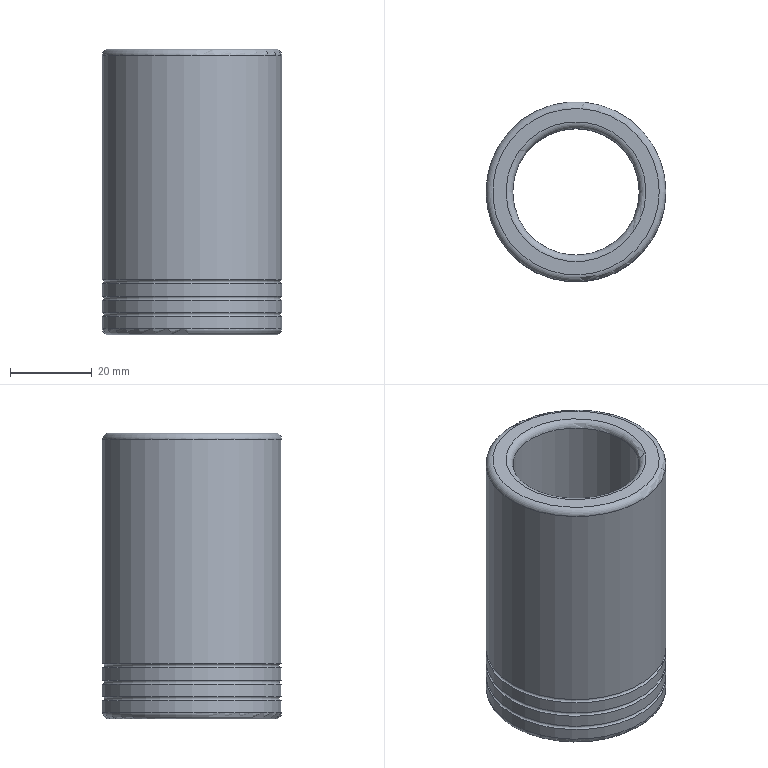Part | STEP file | 1 solid | 14 faces | box 44 x 44 x 70 mm | volume 53175 mm3 | torus 7 | cylinder 5 | plane 2 | commonest cylinder face diameters 44 x4 31 x1
STEP:
#1=CARTESIAN_POINT('',(0.,0.,0.));
#2=DIRECTION('',(0.,0.,1.));
#3=DIRECTION('',(1.,0.,0.));
#4=AXIS2_PLACEMENT_3D('',#1,#2,#3);
#5=CARTESIAN_POINT('',(1551.747,289.48,-77.006));
#6=VERTEX_POINT('',#5);
#7=CARTESIAN_POINT('',(1536.247,289.48,-77.006));
#8=DIRECTION('',(0.,0.,1.));
#9=DIRECTION('',(1.,0.,0.));
#10=AXIS2_PLACEMENT_3D('',#7,#8,#9);
#11=CIRCLE('',#10,15.5);
#12=CARTESIAN_POINT('',(1536.247,289.48,-125.381));
#13=DIRECTION('',(0.,0.,1.));
#14=DIRECTION('',(1.,0.,0.));
#15=AXIS2_PLACEMENT_3D('',#12,#13,#14);
#16=CYLINDRICAL_SURFACE('',#15,15.5);
#17=CARTESIAN_POINT('',(0.,48.375));
#18=DIRECTION('',(1.,0.));
#19=VECTOR('',#18,1.);
#20=LINE('',#17,#19);
#21=(GEOMETRIC_REPRESENTATION_CONTEXT(2)PARAMETRIC_REPRESENTATION_CONTEXT()REPRESENTATION_CONTEXT('',''));
#22=DEFINITIONAL_REPRESENTATION('',(#20),#21);
#23=PCURVE('',#16,#22);
#24=CARTESIAN_POINT('',(1536.247,289.48,-77.006));
#25=DIRECTION('',(0.,0.,1.));
#26=DIRECTION('',(1.,0.,0.));
#27=AXIS2_PLACEMENT_3D('',#24,#25,#26);
#28=TOROIDAL_SURFACE('',#27,17.125,1.625);
#29=CARTESIAN_POINT('',(0.,9.425));
#30=DIRECTION('',(1.,0.));
#31=VECTOR('',#30,1.);
#32=LINE('',#29,#31);
#33=(GEOMETRIC_REPRESENTATION_CONTEXT(2)PARAMETRIC_REPRESENTATION_CONTEXT()REPRESENTATION_CONTEXT('',''));
#34=DEFINITIONAL_REPRESENTATION('',(#32),#33);
#35=PCURVE('',#28,#34);
#36=SURFACE_CURVE('',#11,(#23,#35),.PCURVE_S1.);
#37=EDGE_CURVE('',#6,#6,#36,.T.);
#38=ORIENTED_EDGE('',*,*,#37,.F.);
#39=CARTESIAN_POINT('',(1551.747,289.48,-143.756));
#40=VERTEX_POINT('',#39);
#41=CARTESIAN_POINT('',(1551.747,289.48,-143.756));
#42=CARTESIAN_POINT('',(1551.747,289.48,-77.006));
#43=B_SPLINE_CURVE_WITH_KNOTS('',1,(#41,#42),.UNSPECIFIED.,.F.,.F.,(2,2),(-18.375,48.375),.PIECEWISE_BEZIER_KNOTS.);
#44=CARTESIAN_POINT('',(0.,0.));
#45=DIRECTION('',(0.,1.));
#46=VECTOR('',#45,1.);
#47=LINE('',#44,#46);
#48=(GEOMETRIC_REPRESENTATION_CONTEXT(2)PARAMETRIC_REPRESENTATION_CONTEXT()REPRESENTATION_CONTEXT('',''));
#49=DEFINITIONAL_REPRESENTATION('',(#47),#48);
#50=PCURVE('',#16,#49);
#51=CARTESIAN_POINT('',(6.283,0.));
#52=DIRECTION('',(0.,1.));
#53=VECTOR('',#52,1.);
#54=LINE('',#51,#53);
#55=(GEOMETRIC_REPRESENTATION_CONTEXT(2)PARAMETRIC_REPRESENTATION_CONTEXT()REPRESENTATION_CONTEXT('',''));
#56=DEFINITIONAL_REPRESENTATION('',(#54),#55);
#57=PCURVE('',#16,#56);
#58=SEAM_CURVE('',#43,(#50,#57),.PCURVE_S1.);
#59=EDGE_CURVE('',#40,#6,#58,.T.);
#60=ORIENTED_EDGE('',*,*,#59,.F.);
#61=CARTESIAN_POINT('',(1520.747,289.48,-143.756));
#62=VERTEX_POINT('',#61);
#63=CARTESIAN_POINT('',(1536.247,289.48,-143.756));
#64=DIRECTION('',(0.,0.,-1.));
#65=DIRECTION('',(-1.,0.,0.));
#66=AXIS2_PLACEMENT_3D('',#63,#64,#65);
#67=CIRCLE('',#66,15.5);
#68=CARTESIAN_POINT('',(3.142,-18.375));
#69=DIRECTION('',(-1.,0.));
#70=VECTOR('',#69,1.);
#71=LINE('',#68,#70);
#72=(GEOMETRIC_REPRESENTATION_CONTEXT(2)PARAMETRIC_REPRESENTATION_CONTEXT()REPRESENTATION_CONTEXT('',''));
#73=DEFINITIONAL_REPRESENTATION('',(#71),#72);
#74=PCURVE('',#16,#73);
#75=CARTESIAN_POINT('',(1536.247,289.48,-143.756));
#76=DIRECTION('',(0.,0.,-1.));
#77=DIRECTION('',(-1.,0.,0.));
#78=AXIS2_PLACEMENT_3D('',#75,#76,#77);
#79=TOROIDAL_SURFACE('',#78,17.125,1.625);
#80=CARTESIAN_POINT('',(0.,9.425));
#81=DIRECTION('',(1.,0.));
#82=VECTOR('',#81,1.);
#83=LINE('',#80,#82);
#84=(GEOMETRIC_REPRESENTATION_CONTEXT(2)PARAMETRIC_REPRESENTATION_CONTEXT()REPRESENTATION_CONTEXT('',''));
#85=DEFINITIONAL_REPRESENTATION('',(#83),#84);
#86=PCURVE('',#79,#85);
#87=SURFACE_CURVE('',#67,(#74,#86),.PCURVE_S1.);
#88=EDGE_CURVE('',#62,#40,#87,.T.);
#89=ORIENTED_EDGE('',*,*,#88,.F.);
#90=CARTESIAN_POINT('',(1536.247,289.48,-143.756));
#91=DIRECTION('',(0.,0.,-1.));
#92=DIRECTION('',(-1.,0.,0.));
#93=AXIS2_PLACEMENT_3D('',#90,#91,#92);
#94=CIRCLE('',#93,15.5);
#95=CARTESIAN_POINT('',(9.425,-18.375));
#96=DIRECTION('',(-1.,0.));
#97=VECTOR('',#96,1.);
#98=LINE('',#95,#97);
#99=(GEOMETRIC_REPRESENTATION_CONTEXT(2)PARAMETRIC_REPRESENTATION_CONTEXT()REPRESENTATION_CONTEXT('',''));
#100=DEFINITIONAL_REPRESENTATION('',(#98),#99);
#101=PCURVE('',#16,#100);
#102=CARTESIAN_POINT('',(0.,9.425));
#103=DIRECTION('',(1.,0.));
#104=VECTOR('',#103,1.);
#105=LINE('',#102,#104);
#106=(GEOMETRIC_REPRESENTATION_CONTEXT(2)PARAMETRIC_REPRESENTATION_CONTEXT()REPRESENTATION_CONTEXT('',''));
#107=DEFINITIONAL_REPRESENTATION('',(#105),#106);
#108=PCURVE('',#79,#107);
#109=SURFACE_CURVE('',#94,(#101,#108),.PCURVE_S1.);
#110=EDGE_CURVE('',#40,#62,#109,.T.);
#111=ORIENTED_EDGE('',*,*,#110,.F.);
#112=ORIENTED_EDGE('',*,*,#59,.T.);
#113=EDGE_LOOP('',(#38,#60,#89,#111,#112));
#114=FACE_BOUND('',#113,.F.);
#115=ADVANCED_FACE('',(#114),#16,.F.);
#116=CARTESIAN_POINT('',(1553.372,289.48,-75.381));
#117=VERTEX_POINT('',#116);
#118=CARTESIAN_POINT('',(1536.247,289.48,-75.381));
#119=DIRECTION('',(0.,0.,-1.));
#120=DIRECTION('',(1.,0.,0.));
#121=AXIS2_PLACEMENT_3D('',#118,#119,#120);
#122=CIRCLE('',#121,17.125);
#123=CARTESIAN_POINT('',(1520.747,289.48,-75.381));
#124=DIRECTION('',(0.,0.,1.));
#125=DIRECTION('',(1.,0.,0.));
#126=AXIS2_PLACEMENT_3D('',#123,#124,#125);
#127=PLANE('',#126);
#128=CARTESIAN_POINT('',(32.625,0.));
#129=CARTESIAN_POINT('',(32.625,-29.661));
#130=CARTESIAN_POINT('',(6.938,-14.831));
#131=CARTESIAN_POINT('',(-18.75,0.));
#132=CARTESIAN_POINT('',(6.938,14.831));
#133=CARTESIAN_POINT('',(32.625,29.661));
#134=CARTESIAN_POINT('',(32.625,0.));
#135=(BOUNDED_CURVE()B_SPLINE_CURVE(2,(#128,#129,#130,#131,#132,#133,#134),.UNSPECIFIED.,.T.,.F.)B_SPLINE_CURVE_WITH_KNOTS((1,2,2,2,2,1),(-2.094,0.,2.094,4.189,6.283,8.378),.UNSPECIFIED.)CURVE()GEOMETRIC_REPRESENTATION_ITEM()RATIONAL_B_SPLINE_CURVE((1.,0.5,1.,0.5,1.,0.5,1.))REPRESENTATION_ITEM(''));
#136=(GEOMETRIC_REPRESENTATION_CONTEXT(2)PARAMETRIC_REPRESENTATION_CONTEXT()REPRESENTATION_CONTEXT('',''));
#137=DEFINITIONAL_REPRESENTATION('',(#135),#136);
#138=PCURVE('',#127,#137);
#139=CARTESIAN_POINT('',(6.283,7.854));
#140=DIRECTION('',(-1.,0.));
#141=VECTOR('',#140,1.);
#142=LINE('',#139,#141);
#143=(GEOMETRIC_REPRESENTATION_CONTEXT(2)PARAMETRIC_REPRESENTATION_CONTEXT()REPRESENTATION_CONTEXT('',''));
#144=DEFINITIONAL_REPRESENTATION('',(#142),#143);
#145=PCURVE('',#28,#144);
#146=SURFACE_CURVE('',#122,(#138,#145),.PCURVE_S1.);
#147=EDGE_CURVE('',#117,#117,#146,.T.);
#148=ORIENTED_EDGE('',*,*,#147,.T.);
#149=EDGE_LOOP('',(#148));
#150=FACE_BOUND('',#149,.T.);
#151=CARTESIAN_POINT('',(1556.622,289.48,-75.381));
#152=VERTEX_POINT('',#151);
#153=CARTESIAN_POINT('',(1536.247,289.48,-75.381));
#154=DIRECTION('',(0.,0.,1.));
#155=DIRECTION('',(1.,0.,0.));
#156=AXIS2_PLACEMENT_3D('',#153,#154,#155);
#157=CIRCLE('',#156,20.375);
#158=CARTESIAN_POINT('',(15.5,0.));
#159=DIRECTION('',(1.,0.));
#160=AXIS2_PLACEMENT_2D('',#158,#159);
#161=CIRCLE('',#160,20.375);
#162=(GEOMETRIC_REPRESENTATION_CONTEXT(2)PARAMETRIC_REPRESENTATION_CONTEXT()REPRESENTATION_CONTEXT('',''));
#163=DEFINITIONAL_REPRESENTATION('',(#161),#162);
#164=PCURVE('',#127,#163);
#165=CARTESIAN_POINT('',(1536.247,289.48,-77.006));
#166=DIRECTION('',(0.,0.,1.));
#167=DIRECTION('',(1.,0.,0.));
#168=AXIS2_PLACEMENT_3D('',#165,#166,#167);
#169=TOROIDAL_SURFACE('',#168,20.375,1.625);
#170=CARTESIAN_POINT('',(0.,7.854));
#171=DIRECTION('',(1.,0.));
#172=VECTOR('',#171,1.);
#173=LINE('',#170,#172);
#174=(GEOMETRIC_REPRESENTATION_CONTEXT(2)PARAMETRIC_REPRESENTATION_CONTEXT()REPRESENTATION_CONTEXT('',''));
#175=DEFINITIONAL_REPRESENTATION('',(#173),#174);
#176=PCURVE('',#169,#175);
#177=SURFACE_CURVE('',#157,(#164,#176),.PCURVE_S1.);
#178=EDGE_CURVE('',#152,#152,#177,.T.);
#179=ORIENTED_EDGE('',*,*,#178,.T.);
#180=EDGE_LOOP('',(#179));
#181=FACE_BOUND('',#180,.T.);
#182=ADVANCED_FACE('',(#150,#181),#127,.T.);
#183=CARTESIAN_POINT('',(1558.247,289.48,-77.006));
#184=VERTEX_POINT('',#183);
#185=CARTESIAN_POINT('',(1536.247,289.48,-77.006));
#186=DIRECTION('',(0.,0.,-1.));
#187=DIRECTION('',(1.,0.,0.));
#188=AXIS2_PLACEMENT_3D('',#185,#186,#187);
#189=CIRCLE('',#188,22.);
#190=CARTESIAN_POINT('',(1536.247,289.48,-125.381));
#191=DIRECTION('',(0.,0.,1.));
#192=DIRECTION('',(1.,0.,0.));
#193=AXIS2_PLACEMENT_3D('',#190,#191,#192);
#194=CYLINDRICAL_SURFACE('',#193,22.);
#195=CARTESIAN_POINT('',(6.283,48.375));
#196=DIRECTION('',(-1.,0.));
#197=VECTOR('',#196,1.);
#198=LINE('',#195,#197);
#199=(GEOMETRIC_REPRESENTATION_CONTEXT(2)PARAMETRIC_REPRESENTATION_CONTEXT()REPRESENTATION_CONTEXT('',''));
#200=DEFINITIONAL_REPRESENTATION('',(#198),#199);
#201=PCURVE('',#194,#200);
#202=CARTESIAN_POINT('',(6.283,6.283));
#203=DIRECTION('',(-1.,0.));
#204=VECTOR('',#203,1.);
#205=LINE('',#202,#204);
#206=(GEOMETRIC_REPRESENTATION_CONTEXT(2)PARAMETRIC_REPRESENTATION_CONTEXT()REPRESENTATION_CONTEXT('',''));
#207=DEFINITIONAL_REPRESENTATION('',(#205),#206);
#208=PCURVE('',#169,#207);
#209=SURFACE_CURVE('',#189,(#201,#208),.PCURVE_S1.);
#210=EDGE_CURVE('',#184,#184,#209,.T.);
#211=ORIENTED_EDGE('',*,*,#210,.T.);
#212=CARTESIAN_POINT('',(1558.247,289.48,-131.881));
#213=VERTEX_POINT('',#212);
#214=CARTESIAN_POINT('',(1558.247,289.48,-131.881));
#215=CARTESIAN_POINT('',(1558.247,289.48,-77.006));
#216=B_SPLINE_CURVE_WITH_KNOTS('',1,(#214,#215),.UNSPECIFIED.,.F.,.F.,(2,2),(-6.5,48.375),.PIECEWISE_BEZIER_KNOTS.);
#217=CARTESIAN_POINT('',(0.,0.));
#218=DIRECTION('',(0.,1.));
#219=VECTOR('',#218,1.);
#220=LINE('',#217,#219);
#221=(GEOMETRIC_REPRESENTATION_CONTEXT(2)PARAMETRIC_REPRESENTATION_CONTEXT()REPRESENTATION_CONTEXT('',''));
#222=DEFINITIONAL_REPRESENTATION('',(#220),#221);
#223=PCURVE('',#194,#222);
#224=CARTESIAN_POINT('',(6.283,0.));
#225=DIRECTION('',(0.,1.));
#226=VECTOR('',#225,1.);
#227=LINE('',#224,#226);
#228=(GEOMETRIC_REPRESENTATION_CONTEXT(2)PARAMETRIC_REPRESENTATION_CONTEXT()REPRESENTATION_CONTEXT('',''));
#229=DEFINITIONAL_REPRESENTATION('',(#227),#228);
#230=PCURVE('',#194,#229);
#231=SEAM_CURVE('',#216,(#223,#230),.PCURVE_S1.);
#232=EDGE_CURVE('',#213,#184,#231,.T.);
#233=ORIENTED_EDGE('',*,*,#232,.F.);
#234=CARTESIAN_POINT('',(1536.247,289.48,-131.881));
#235=DIRECTION('',(0.,0.,1.));
#236=DIRECTION('',(1.,0.,0.));
#237=AXIS2_PLACEMENT_3D('',#234,#235,#236);
#238=CIRCLE('',#237,22.);
#239=CARTESIAN_POINT('',(0.,-6.5));
#240=DIRECTION('',(1.,0.));
#241=VECTOR('',#240,1.);
#242=LINE('',#239,#241);
#243=(GEOMETRIC_REPRESENTATION_CONTEXT(2)PARAMETRIC_REPRESENTATION_CONTEXT()REPRESENTATION_CONTEXT('',''));
#244=DEFINITIONAL_REPRESENTATION('',(#242),#243);
#245=PCURVE('',#194,#244);
#246=CARTESIAN_POINT('',(1536.247,289.48,-132.381));
#247=DIRECTION('',(0.,0.,1.));
#248=DIRECTION('',(1.,0.,0.));
#249=AXIS2_PLACEMENT_3D('',#246,#247,#248);
#250=TOROIDAL_SURFACE('',#249,22.,0.5);
#251=CARTESIAN_POINT('',(0.,1.571));
#252=DIRECTION('',(1.,0.));
#253=VECTOR('',#252,1.);
#254=LINE('',#251,#253);
#255=(GEOMETRIC_REPRESENTATION_CONTEXT(2)PARAMETRIC_REPRESENTATION_CONTEXT()REPRESENTATION_CONTEXT('',''));
#256=DEFINITIONAL_REPRESENTATION('',(#254),#255);
#257=PCURVE('',#250,#256);
#258=SURFACE_CURVE('',#238,(#245,#257),.PCURVE_S1.);
#259=EDGE_CURVE('',#213,#213,#258,.T.);
#260=ORIENTED_EDGE('',*,*,#259,.T.);
#261=ORIENTED_EDGE('',*,*,#232,.T.);
#262=EDGE_LOOP('',(#211,#233,#260,#261));
#263=FACE_BOUND('',#262,.T.);
#264=ADVANCED_FACE('',(#263),#194,.T.);
#265=CARTESIAN_POINT('',(1558.247,289.48,-132.881));
#266=VERTEX_POINT('',#265);
#267=CARTESIAN_POINT('',(1536.247,289.48,-132.881));
#268=DIRECTION('',(0.,0.,1.));
#269=DIRECTION('',(1.,0.,0.));
#270=AXIS2_PLACEMENT_3D('',#267,#268,#269);
#271=CIRCLE('',#270,22.);
#272=CARTESIAN_POINT('',(0.,4.712));
#273=DIRECTION('',(1.,0.));
#274=VECTOR('',#273,1.);
#275=LINE('',#272,#274);
#276=(GEOMETRIC_REPRESENTATION_CONTEXT(2)PARAMETRIC_REPRESENTATION_CONTEXT()REPRESENTATION_CONTEXT('',''));
#277=DEFINITIONAL_REPRESENTATION('',(#275),#276);
#278=PCURVE('',#250,#277);
#279=CARTESIAN_POINT('',(1536.247,289.48,-125.381));
#280=DIRECTION('',(0.,0.,1.));
#281=DIRECTION('',(1.,0.,0.));
#282=AXIS2_PLACEMENT_3D('',#279,#280,#281);
#283=CYLINDRICAL_SURFACE('',#282,22.);
#284=CARTESIAN_POINT('',(0.,-7.5));
#285=DIRECTION('',(1.,0.));
#286=VECTOR('',#285,1.);
#287=LINE('',#284,#286);
#288=(GEOMETRIC_REPRESENTATION_CONTEXT(2)PARAMETRIC_REPRESENTATION_CONTEXT()REPRESENTATION_CONTEXT('',''));
#289=DEFINITIONAL_REPRESENTATION('',(#287),#288);
#290=PCURVE('',#283,#289);
#291=SURFACE_CURVE('',#271,(#278,#290),.PCURVE_S1.);
#292=EDGE_CURVE('',#266,#266,#291,.T.);
#293=ORIENTED_EDGE('',*,*,#292,.F.);
#294=CARTESIAN_POINT('',(1558.247,289.48,-131.881));
#295=CARTESIAN_POINT('',(1558.023,289.48,-131.881));
#296=CARTESIAN_POINT('',(1557.799,289.48,-131.998));
#297=CARTESIAN_POINT('',(1557.647,289.48,-132.233));
#298=CARTESIAN_POINT('',(1557.647,289.48,-132.529));
#299=CARTESIAN_POINT('',(1557.799,289.48,-132.763));
#300=CARTESIAN_POINT('',(1558.023,289.48,-132.881));
#301=CARTESIAN_POINT('',(1558.247,289.48,-132.881));
#302=B_SPLINE_CURVE_WITH_KNOTS('',7,(#294,#295,#296,#297,#298,#299,#300,#301),.UNSPECIFIED.,.F.,.F.,(8,8),(1.571,4.712),.PIECEWISE_BEZIER_KNOTS.);
#303=CARTESIAN_POINT('',(0.,0.));
#304=DIRECTION('',(0.,1.));
#305=VECTOR('',#304,1.);
#306=LINE('',#303,#305);
#307=(GEOMETRIC_REPRESENTATION_CONTEXT(2)PARAMETRIC_REPRESENTATION_CONTEXT()REPRESENTATION_CONTEXT('',''));
#308=DEFINITIONAL_REPRESENTATION('',(#306),#307);
#309=PCURVE('',#250,#308);
#310=CARTESIAN_POINT('',(6.283,0.));
#311=DIRECTION('',(0.,1.));
#312=VECTOR('',#311,1.);
#313=LINE('',#310,#312);
#314=(GEOMETRIC_REPRESENTATION_CONTEXT(2)PARAMETRIC_REPRESENTATION_CONTEXT()REPRESENTATION_CONTEXT('',''));
#315=DEFINITIONAL_REPRESENTATION('',(#313),#314);
#316=PCURVE('',#250,#315);
#317=SEAM_CURVE('',#302,(#309,#316),.PCURVE_S1.);
#318=EDGE_CURVE('',#213,#266,#317,.T.);
#319=ORIENTED_EDGE('',*,*,#318,.F.);
#320=ORIENTED_EDGE('',*,*,#259,.T.);
#321=ORIENTED_EDGE('',*,*,#318,.T.);
#322=EDGE_LOOP('',(#293,#319,#320,#321));
#323=FACE_BOUND('',#322,.F.);
#324=ADVANCED_FACE('',(#323),#250,.F.);
#325=CARTESIAN_POINT('',(1558.247,289.48,-135.881));
#326=VERTEX_POINT('',#325);
#327=CARTESIAN_POINT('',(1536.247,289.48,-135.881));
#328=DIRECTION('',(0.,0.,1.));
#329=DIRECTION('',(1.,0.,0.));
#330=AXIS2_PLACEMENT_3D('',#327,#328,#329);
#331=CIRCLE('',#330,22.);
#332=CARTESIAN_POINT('',(0.,-10.5));
#333=DIRECTION('',(1.,0.));
#334=VECTOR('',#333,1.);
#335=LINE('',#332,#334);
#336=(GEOMETRIC_REPRESENTATION_CONTEXT(2)PARAMETRIC_REPRESENTATION_CONTEXT()REPRESENTATION_CONTEXT('',''));
#337=DEFINITIONAL_REPRESENTATION('',(#335),#336);
#338=PCURVE('',#283,#337);
#339=CARTESIAN_POINT('',(1536.247,289.48,-136.381));
#340=DIRECTION('',(0.,0.,1.));
#341=DIRECTION('',(1.,0.,0.));
#342=AXIS2_PLACEMENT_3D('',#339,#340,#341);
#343=TOROIDAL_SURFACE('',#342,22.,0.5);
#344=CARTESIAN_POINT('',(0.,1.571));
#345=DIRECTION('',(1.,0.));
#346=VECTOR('',#345,1.);
#347=LINE('',#344,#346);
#348=(GEOMETRIC_REPRESENTATION_CONTEXT(2)PARAMETRIC_REPRESENTATION_CONTEXT()REPRESENTATION_CONTEXT('',''));
#349=DEFINITIONAL_REPRESENTATION('',(#347),#348);
#350=PCURVE('',#343,#349);
#351=SURFACE_CURVE('',#331,(#338,#350),.PCURVE_S1.);
#352=EDGE_CURVE('',#326,#326,#351,.T.);
#353=ORIENTED_EDGE('',*,*,#352,.T.);
#354=CARTESIAN_POINT('',(1558.247,289.48,-135.881));
#355=CARTESIAN_POINT('',(1558.247,289.48,-132.881));
#356=B_SPLINE_CURVE_WITH_KNOTS('',1,(#354,#355),.UNSPECIFIED.,.F.,.F.,(2,2),(-10.5,-7.5),.PIECEWISE_BEZIER_KNOTS.);
#357=CARTESIAN_POINT('',(6.283,0.));
#358=DIRECTION('',(0.,1.));
#359=VECTOR('',#358,1.);
#360=LINE('',#357,#359);
#361=(GEOMETRIC_REPRESENTATION_CONTEXT(2)PARAMETRIC_REPRESENTATION_CONTEXT()REPRESENTATION_CONTEXT('',''));
#362=DEFINITIONAL_REPRESENTATION('',(#360),#361);
#363=PCURVE('',#283,#362);
#364=CARTESIAN_POINT('',(0.,0.));
#365=DIRECTION('',(0.,1.));
#366=VECTOR('',#365,1.);
#367=LINE('',#364,#366);
#368=(GEOMETRIC_REPRESENTATION_CONTEXT(2)PARAMETRIC_REPRESENTATION_CONTEXT()REPRESENTATION_CONTEXT('',''));
#369=DEFINITIONAL_REPRESENTATION('',(#367),#368);
#370=PCURVE('',#283,#369);
#371=SEAM_CURVE('',#356,(#363,#370),.PCURVE_S1.);
#372=EDGE_CURVE('',#326,#266,#371,.T.);
#373=ORIENTED_EDGE('',*,*,#372,.T.);
#374=ORIENTED_EDGE('',*,*,#292,.F.);
#375=ORIENTED_EDGE('',*,*,#372,.F.);
#376=EDGE_LOOP('',(#353,#373,#374,#375));
#377=FACE_BOUND('',#376,.T.);
#378=ADVANCED_FACE('',(#377),#283,.T.);
#379=CARTESIAN_POINT('',(1558.247,289.48,-136.881));
#380=VERTEX_POINT('',#379);
#381=CARTESIAN_POINT('',(1536.247,289.48,-136.881));
#382=DIRECTION('',(0.,0.,1.));
#383=DIRECTION('',(1.,0.,0.));
#384=AXIS2_PLACEMENT_3D('',#381,#382,#383);
#385=CIRCLE('',#384,22.);
#386=CARTESIAN_POINT('',(0.,4.712));
#387=DIRECTION('',(1.,0.));
#388=VECTOR('',#387,1.);
#389=LINE('',#386,#388);
#390=(GEOMETRIC_REPRESENTATION_CONTEXT(2)PARAMETRIC_REPRESENTATION_CONTEXT()REPRESENTATION_CONTEXT('',''));
#391=DEFINITIONAL_REPRESENTATION('',(#389),#390);
#392=PCURVE('',#343,#391);
#393=CARTESIAN_POINT('',(1536.247,289.48,-125.381));
#394=DIRECTION('',(0.,0.,1.));
#395=DIRECTION('',(1.,0.,0.));
#396=AXIS2_PLACEMENT_3D('',#393,#394,#395);
#397=CYLINDRICAL_SURFACE('',#396,22.);
#398=CARTESIAN_POINT('',(0.,-11.5));
#399=DIRECTION('',(1.,0.));
#400=VECTOR('',#399,1.);
#401=LINE('',#398,#400);
#402=(GEOMETRIC_REPRESENTATION_CONTEXT(2)PARAMETRIC_REPRESENTATION_CONTEXT()REPRESENTATION_CONTEXT('',''));
#403=DEFINITIONAL_REPRESENTATION('',(#401),#402);
#404=PCURVE('',#397,#403);
#405=SURFACE_CURVE('',#385,(#392,#404),.PCURVE_S1.);
#406=EDGE_CURVE('',#380,#380,#405,.T.);
#407=ORIENTED_EDGE('',*,*,#406,.F.);
#408=CARTESIAN_POINT('',(1558.247,289.48,-135.881));
#409=CARTESIAN_POINT('',(1558.023,289.48,-135.881));
#410=CARTESIAN_POINT('',(1557.799,289.48,-135.998));
#411=CARTESIAN_POINT('',(1557.647,289.48,-136.233));
#412=CARTESIAN_POINT('',(1557.647,289.48,-136.529));
#413=CARTESIAN_POINT('',(1557.799,289.48,-136.763));
#414=CARTESIAN_POINT('',(1558.023,289.48,-136.881));
#415=CARTESIAN_POINT('',(1558.247,289.48,-136.881));
#416=B_SPLINE_CURVE_WITH_KNOTS('',7,(#408,#409,#410,#411,#412,#413,#414,#415),.UNSPECIFIED.,.F.,.F.,(8,8),(1.571,4.712),.PIECEWISE_BEZIER_KNOTS.);
#417=CARTESIAN_POINT('',(0.,0.));
#418=DIRECTION('',(0.,1.));
#419=VECTOR('',#418,1.);
#420=LINE('',#417,#419);
#421=(GEOMETRIC_REPRESENTATION_CONTEXT(2)PARAMETRIC_REPRESENTATION_CONTEXT()REPRESENTATION_CONTEXT('',''));
#422=DEFINITIONAL_REPRESENTATION('',(#420),#421);
#423=PCURVE('',#343,#422);
#424=CARTESIAN_POINT('',(6.283,0.));
#425=DIRECTION('',(0.,1.));
#426=VECTOR('',#425,1.);
#427=LINE('',#424,#426);
#428=(GEOMETRIC_REPRESENTATION_CONTEXT(2)PARAMETRIC_REPRESENTATION_CONTEXT()REPRESENTATION_CONTEXT('',''));
#429=DEFINITIONAL_REPRESENTATION('',(#427),#428);
#430=PCURVE('',#343,#429);
#431=SEAM_CURVE('',#416,(#423,#430),.PCURVE_S1.);
#432=EDGE_CURVE('',#326,#380,#431,.T.);
#433=ORIENTED_EDGE('',*,*,#432,.F.);
#434=ORIENTED_EDGE('',*,*,#352,.T.);
#435=ORIENTED_EDGE('',*,*,#432,.T.);
#436=EDGE_LOOP('',(#407,#433,#434,#435));
#437=FACE_BOUND('',#436,.F.);
#438=ADVANCED_FACE('',(#437),#343,.F.);
#439=CARTESIAN_POINT('',(1558.247,289.48,-139.881));
#440=VERTEX_POINT('',#439);
#441=CARTESIAN_POINT('',(1536.247,289.48,-139.881));
#442=DIRECTION('',(0.,0.,1.));
#443=DIRECTION('',(1.,0.,0.));
#444=AXIS2_PLACEMENT_3D('',#441,#442,#443);
#445=CIRCLE('',#444,22.);
#446=CARTESIAN_POINT('',(0.,-14.5));
#447=DIRECTION('',(1.,0.));
#448=VECTOR('',#447,1.);
#449=LINE('',#446,#448);
#450=(GEOMETRIC_REPRESENTATION_CONTEXT(2)PARAMETRIC_REPRESENTATION_CONTEXT()REPRESENTATION_CONTEXT('',''));
#451=DEFINITIONAL_REPRESENTATION('',(#449),#450);
#452=PCURVE('',#397,#451);
#453=CARTESIAN_POINT('',(1536.247,289.48,-140.381));
#454=DIRECTION('',(0.,0.,1.));
#455=DIRECTION('',(1.,0.,0.));
#456=AXIS2_PLACEMENT_3D('',#453,#454,#455);
#457=TOROIDAL_SURFACE('',#456,22.,0.5);
#458=CARTESIAN_POINT('',(0.,1.571));
#459=DIRECTION('',(1.,0.));
#460=VECTOR('',#459,1.);
#461=LINE('',#458,#460);
#462=(GEOMETRIC_REPRESENTATION_CONTEXT(2)PARAMETRIC_REPRESENTATION_CONTEXT()REPRESENTATION_CONTEXT('',''));
#463=DEFINITIONAL_REPRESENTATION('',(#461),#462);
#464=PCURVE('',#457,#463);
#465=SURFACE_CURVE('',#445,(#452,#464),.PCURVE_S1.);
#466=EDGE_CURVE('',#440,#440,#465,.T.);
#467=ORIENTED_EDGE('',*,*,#466,.T.);
#468=CARTESIAN_POINT('',(1558.247,289.48,-139.881));
#469=CARTESIAN_POINT('',(1558.247,289.48,-136.881));
#470=B_SPLINE_CURVE_WITH_KNOTS('',1,(#468,#469),.UNSPECIFIED.,.F.,.F.,(2,2),(-14.5,-11.5),.PIECEWISE_BEZIER_KNOTS.);
#471=CARTESIAN_POINT('',(6.283,0.));
#472=DIRECTION('',(0.,1.));
#473=VECTOR('',#472,1.);
#474=LINE('',#471,#473);
#475=(GEOMETRIC_REPRESENTATION_CONTEXT(2)PARAMETRIC_REPRESENTATION_CONTEXT()REPRESENTATION_CONTEXT('',''));
#476=DEFINITIONAL_REPRESENTATION('',(#474),#475);
#477=PCURVE('',#397,#476);
#478=CARTESIAN_POINT('',(0.,0.));
#479=DIRECTION('',(0.,1.));
#480=VECTOR('',#479,1.);
#481=LINE('',#478,#480);
#482=(GEOMETRIC_REPRESENTATION_CONTEXT(2)PARAMETRIC_REPRESENTATION_CONTEXT()REPRESENTATION_CONTEXT('',''));
#483=DEFINITIONAL_REPRESENTATION('',(#481),#482);
#484=PCURVE('',#397,#483);
#485=SEAM_CURVE('',#470,(#477,#484),.PCURVE_S1.);
#486=EDGE_CURVE('',#440,#380,#485,.T.);
#487=ORIENTED_EDGE('',*,*,#486,.T.);
#488=ORIENTED_EDGE('',*,*,#406,.F.);
#489=ORIENTED_EDGE('',*,*,#486,.F.);
#490=EDGE_LOOP('',(#467,#487,#488,#489));
#491=FACE_BOUND('',#490,.T.);
#492=ADVANCED_FACE('',(#491),#397,.T.);
#493=CARTESIAN_POINT('',(1558.247,289.48,-140.881));
#494=VERTEX_POINT('',#493);
#495=CARTESIAN_POINT('',(1536.247,289.48,-140.881));
#496=DIRECTION('',(0.,0.,1.));
#497=DIRECTION('',(1.,0.,0.));
#498=AXIS2_PLACEMENT_3D('',#495,#496,#497);
#499=CIRCLE('',#498,22.);
#500=CARTESIAN_POINT('',(0.,4.712));
#501=DIRECTION('',(1.,0.));
#502=VECTOR('',#501,1.);
#503=LINE('',#500,#502);
#504=(GEOMETRIC_REPRESENTATION_CONTEXT(2)PARAMETRIC_REPRESENTATION_CONTEXT()REPRESENTATION_CONTEXT('',''));
#505=DEFINITIONAL_REPRESENTATION('',(#503),#504);
#506=PCURVE('',#457,#505);
#507=CARTESIAN_POINT('',(1536.247,289.48,-125.381));
#508=DIRECTION('',(0.,0.,1.));
#509=DIRECTION('',(1.,0.,0.));
#510=AXIS2_PLACEMENT_3D('',#507,#508,#509);
#511=CYLINDRICAL_SURFACE('',#510,22.);
#512=CARTESIAN_POINT('',(0.,-15.5));
#513=DIRECTION('',(1.,0.));
#514=VECTOR('',#513,1.);
#515=LINE('',#512,#514);
#516=(GEOMETRIC_REPRESENTATION_CONTEXT(2)PARAMETRIC_REPRESENTATION_CONTEXT()REPRESENTATION_CONTEXT('',''));
#517=DEFINITIONAL_REPRESENTATION('',(#515),#516);
#518=PCURVE('',#511,#517);
#519=SURFACE_CURVE('',#499,(#506,#518),.PCURVE_S1.);
#520=EDGE_CURVE('',#494,#494,#519,.T.);
#521=ORIENTED_EDGE('',*,*,#520,.F.);
#522=CARTESIAN_POINT('',(1558.247,289.48,-139.881));
#523=CARTESIAN_POINT('',(1558.023,289.48,-139.881));
#524=CARTESIAN_POINT('',(1557.799,289.48,-139.998));
#525=CARTESIAN_POINT('',(1557.647,289.48,-140.233));
#526=CARTESIAN_POINT('',(1557.647,289.48,-140.529));
#527=CARTESIAN_POINT('',(1557.799,289.48,-140.763));
#528=CARTESIAN_POINT('',(1558.023,289.48,-140.881));
#529=CARTESIAN_POINT('',(1558.247,289.48,-140.881));
#530=B_SPLINE_CURVE_WITH_KNOTS('',7,(#522,#523,#524,#525,#526,#527,#528,#529),.UNSPECIFIED.,.F.,.F.,(8,8),(1.571,4.712),.PIECEWISE_BEZIER_KNOTS.);
#531=CARTESIAN_POINT('',(0.,0.));
#532=DIRECTION('',(0.,1.));
#533=VECTOR('',#532,1.);
#534=LINE('',#531,#533);
#535=(GEOMETRIC_REPRESENTATION_CONTEXT(2)PARAMETRIC_REPRESENTATION_CONTEXT()REPRESENTATION_CONTEXT('',''));
#536=DEFINITIONAL_REPRESENTATION('',(#534),#535);
#537=PCURVE('',#457,#536);
#538=CARTESIAN_POINT('',(6.283,0.));
#539=DIRECTION('',(0.,1.));
#540=VECTOR('',#539,1.);
#541=LINE('',#538,#540);
#542=(GEOMETRIC_REPRESENTATION_CONTEXT(2)PARAMETRIC_REPRESENTATION_CONTEXT()REPRESENTATION_CONTEXT('',''));
#543=DEFINITIONAL_REPRESENTATION('',(#541),#542);
#544=PCURVE('',#457,#543);
#545=SEAM_CURVE('',#530,(#537,#544),.PCURVE_S1.);
#546=EDGE_CURVE('',#440,#494,#545,.T.);
#547=ORIENTED_EDGE('',*,*,#546,.F.);
#548=ORIENTED_EDGE('',*,*,#466,.T.);
#549=ORIENTED_EDGE('',*,*,#546,.T.);
#550=EDGE_LOOP('',(#521,#547,#548,#549));
#551=FACE_BOUND('',#550,.F.);
#552=ADVANCED_FACE('',(#551),#457,.F.);
#553=CARTESIAN_POINT('',(1514.247,289.48,-143.756));
#554=VERTEX_POINT('',#553);
#555=CARTESIAN_POINT('',(1558.247,289.48,-143.756));
#556=VERTEX_POINT('',#555);
#557=CARTESIAN_POINT('',(1536.247,289.48,-143.756));
#558=DIRECTION('',(0.,0.,1.));
#559=DIRECTION('',(-1.,0.,0.));
#560=AXIS2_PLACEMENT_3D('',#557,#558,#559);
#561=CIRCLE('',#560,22.);
#562=CARTESIAN_POINT('',(3.142,-18.375));
#563=DIRECTION('',(1.,0.));
#564=VECTOR('',#563,1.);
#565=LINE('',#562,#564);
#566=(GEOMETRIC_REPRESENTATION_CONTEXT(2)PARAMETRIC_REPRESENTATION_CONTEXT()REPRESENTATION_CONTEXT('',''));
#567=DEFINITIONAL_REPRESENTATION('',(#565),#566);
#568=PCURVE('',#511,#567);
#569=CARTESIAN_POINT('',(1536.247,289.48,-143.756));
#570=DIRECTION('',(0.,0.,-1.));
#571=DIRECTION('',(-1.,0.,0.));
#572=AXIS2_PLACEMENT_3D('',#569,#570,#571);
#573=TOROIDAL_SURFACE('',#572,20.375,1.625);
#574=CARTESIAN_POINT('',(6.283,6.283));
#575=DIRECTION('',(-1.,0.));
#576=VECTOR('',#575,1.);
#577=LINE('',#574,#576);
#578=(GEOMETRIC_REPRESENTATION_CONTEXT(2)PARAMETRIC_REPRESENTATION_CONTEXT()REPRESENTATION_CONTEXT('',''));
#579=DEFINITIONAL_REPRESENTATION('',(#577),#578);
#580=PCURVE('',#573,#579);
#581=SURFACE_CURVE('',#561,(#568,#580),.PCURVE_S1.);
#582=EDGE_CURVE('',#554,#556,#581,.T.);
#583=ORIENTED_EDGE('',*,*,#582,.T.);
#584=CARTESIAN_POINT('',(1558.247,289.48,-143.756));
#585=CARTESIAN_POINT('',(1558.247,289.48,-140.881));
#586=B_SPLINE_CURVE_WITH_KNOTS('',1,(#584,#585),.UNSPECIFIED.,.F.,.F.,(2,2),(-18.375,-15.5),.PIECEWISE_BEZIER_KNOTS.);
#587=CARTESIAN_POINT('',(6.283,0.));
#588=DIRECTION('',(0.,1.));
#589=VECTOR('',#588,1.);
#590=LINE('',#587,#589);
#591=(GEOMETRIC_REPRESENTATION_CONTEXT(2)PARAMETRIC_REPRESENTATION_CONTEXT()REPRESENTATION_CONTEXT('',''));
#592=DEFINITIONAL_REPRESENTATION('',(#590),#591);
#593=PCURVE('',#511,#592);
#594=CARTESIAN_POINT('',(0.,0.));
#595=DIRECTION('',(0.,1.));
#596=VECTOR('',#595,1.);
#597=LINE('',#594,#596);
#598=(GEOMETRIC_REPRESENTATION_CONTEXT(2)PARAMETRIC_REPRESENTATION_CONTEXT()REPRESENTATION_CONTEXT('',''));
#599=DEFINITIONAL_REPRESENTATION('',(#597),#598);
#600=PCURVE('',#511,#599);
#601=SEAM_CURVE('',#586,(#593,#600),.PCURVE_S1.);
#602=EDGE_CURVE('',#556,#494,#601,.T.);
#603=ORIENTED_EDGE('',*,*,#602,.T.);
#604=ORIENTED_EDGE('',*,*,#520,.F.);
#605=ORIENTED_EDGE('',*,*,#602,.F.);
#606=CARTESIAN_POINT('',(1536.247,289.48,-143.756));
#607=DIRECTION('',(0.,0.,1.));
#608=DIRECTION('',(-1.,0.,0.));
#609=AXIS2_PLACEMENT_3D('',#606,#607,#608);
#610=CIRCLE('',#609,22.);
#611=CARTESIAN_POINT('',(-3.142,-18.375));
#612=DIRECTION('',(1.,0.));
#613=VECTOR('',#612,1.);
#614=LINE('',#611,#613);
#615=(GEOMETRIC_REPRESENTATION_CONTEXT(2)PARAMETRIC_REPRESENTATION_CONTEXT()REPRESENTATION_CONTEXT('',''));
#616=DEFINITIONAL_REPRESENTATION('',(#614),#615);
#617=PCURVE('',#511,#616);
#618=CARTESIAN_POINT('',(6.283,6.283));
#619=DIRECTION('',(-1.,0.));
#620=VECTOR('',#619,1.);
#621=LINE('',#618,#620);
#622=(GEOMETRIC_REPRESENTATION_CONTEXT(2)PARAMETRIC_REPRESENTATION_CONTEXT()REPRESENTATION_CONTEXT('',''));
#623=DEFINITIONAL_REPRESENTATION('',(#621),#622);
#624=PCURVE('',#573,#623);
#625=SURFACE_CURVE('',#610,(#617,#624),.PCURVE_S1.);
#626=EDGE_CURVE('',#556,#554,#625,.T.);
#627=ORIENTED_EDGE('',*,*,#626,.T.);
#628=EDGE_LOOP('',(#583,#603,#604,#605,#627));
#629=FACE_BOUND('',#628,.T.);
#630=ADVANCED_FACE('',(#629),#511,.T.);
#631=CARTESIAN_POINT('',(1515.872,289.48,-145.381));
#632=VERTEX_POINT('',#631);
#633=CARTESIAN_POINT('',(1536.247,289.48,-145.381));
#634=DIRECTION('',(0.,0.,-1.));
#635=DIRECTION('',(-1.,0.,0.));
#636=AXIS2_PLACEMENT_3D('',#633,#634,#635);
#637=CIRCLE('',#636,20.375);
#638=CARTESIAN_POINT('',(1514.247,289.48,-145.381));
#639=DIRECTION('',(0.,0.,-1.));
#640=DIRECTION('',(-1.,0.,0.));
#641=AXIS2_PLACEMENT_3D('',#638,#639,#640);
#642=PLANE('',#641);
#643=CARTESIAN_POINT('',(-22.,0.));
#644=DIRECTION('',(1.,0.));
#645=AXIS2_PLACEMENT_2D('',#643,#644);
#646=CIRCLE('',#645,20.375);
#647=(GEOMETRIC_REPRESENTATION_CONTEXT(2)PARAMETRIC_REPRESENTATION_CONTEXT()REPRESENTATION_CONTEXT('',''));
#648=DEFINITIONAL_REPRESENTATION('',(#646),#647);
#649=PCURVE('',#642,#648);
#650=CARTESIAN_POINT('',(0.,7.854));
#651=DIRECTION('',(1.,0.));
#652=VECTOR('',#651,1.);
#653=LINE('',#650,#652);
#654=(GEOMETRIC_REPRESENTATION_CONTEXT(2)PARAMETRIC_REPRESENTATION_CONTEXT()REPRESENTATION_CONTEXT('',''));
#655=DEFINITIONAL_REPRESENTATION('',(#653),#654);
#656=PCURVE('',#573,#655);
#657=SURFACE_CURVE('',#637,(#649,#656),.PCURVE_S1.);
#658=EDGE_CURVE('',#632,#632,#657,.T.);
#659=ORIENTED_EDGE('',*,*,#658,.T.);
#660=EDGE_LOOP('',(#659));
#661=FACE_BOUND('',#660,.T.);
#662=CARTESIAN_POINT('',(1519.122,289.48,-145.381));
#663=VERTEX_POINT('',#662);
#664=CARTESIAN_POINT('',(1536.247,289.48,-145.381));
#665=DIRECTION('',(0.,0.,1.));
#666=DIRECTION('',(-1.,0.,0.));
#667=AXIS2_PLACEMENT_3D('',#664,#665,#666);
#668=CIRCLE('',#667,17.125);
#669=CARTESIAN_POINT('',(-4.875,0.));
#670=CARTESIAN_POINT('',(-4.875,-29.661));
#671=CARTESIAN_POINT('',(-30.562,-14.831));
#672=CARTESIAN_POINT('',(-56.25,0.));
#673=CARTESIAN_POINT('',(-30.562,14.831));
#674=CARTESIAN_POINT('',(-4.875,29.661));
#675=CARTESIAN_POINT('',(-4.875,0.));
#676=(BOUNDED_CURVE()B_SPLINE_CURVE(2,(#669,#670,#671,#672,#673,#674,#675),.UNSPECIFIED.,.T.,.F.)B_SPLINE_CURVE_WITH_KNOTS((1,2,2,2,2,1),(-2.094,0.,2.094,4.189,6.283,8.378),.UNSPECIFIED.)CURVE()GEOMETRIC_REPRESENTATION_ITEM()RATIONAL_B_SPLINE_CURVE((1.,0.5,1.,0.5,1.,0.5,1.))REPRESENTATION_ITEM(''));
#677=(GEOMETRIC_REPRESENTATION_CONTEXT(2)PARAMETRIC_REPRESENTATION_CONTEXT()REPRESENTATION_CONTEXT('',''));
#678=DEFINITIONAL_REPRESENTATION('',(#676),#677);
#679=PCURVE('',#642,#678);
#680=CARTESIAN_POINT('',(6.283,7.854));
#681=DIRECTION('',(-1.,0.));
#682=VECTOR('',#681,1.);
#683=LINE('',#680,#682);
#684=(GEOMETRIC_REPRESENTATION_CONTEXT(2)PARAMETRIC_REPRESENTATION_CONTEXT()REPRESENTATION_CONTEXT('',''));
#685=DEFINITIONAL_REPRESENTATION('',(#683),#684);
#686=PCURVE('',#79,#685);
#687=SURFACE_CURVE('',#668,(#679,#686),.PCURVE_S1.);
#688=EDGE_CURVE('',#663,#663,#687,.T.);
#689=ORIENTED_EDGE('',*,*,#688,.T.);
#690=EDGE_LOOP('',(#689));
#691=FACE_BOUND('',#690,.T.);
#692=ADVANCED_FACE('',(#661,#691),#642,.T.);
#693=ORIENTED_EDGE('',*,*,#658,.F.);
#694=CARTESIAN_POINT('',(1514.247,289.48,-143.756));
#695=CARTESIAN_POINT('',(1514.247,289.48,-144.19));
#696=CARTESIAN_POINT('',(1514.385,289.48,-144.613));
#697=CARTESIAN_POINT('',(1514.65,289.48,-144.978));
#698=CARTESIAN_POINT('',(1515.015,289.48,-145.243));
#699=CARTESIAN_POINT('',(1515.438,289.48,-145.381));
#700=CARTESIAN_POINT('',(1515.872,289.48,-145.381));
#701=(BOUNDED_CURVE()B_SPLINE_CURVE(6,(#694,#695,#696,#697,#698,#699,#700),.UNSPECIFIED.,.F.,.F.)B_SPLINE_CURVE_WITH_KNOTS((7,7),(0.,1.571),.PIECEWISE_BEZIER_KNOTS.)CURVE()GEOMETRIC_REPRESENTATION_ITEM()RATIONAL_B_SPLINE_CURVE((1.031,1.01,0.9979,0.994,0.9979,1.01,1.031))REPRESENTATION_ITEM(''));
#702=CARTESIAN_POINT('',(0.,6.283));
#703=DIRECTION('',(0.,1.));
#704=VECTOR('',#703,1.);
#705=LINE('',#702,#704);
#706=(GEOMETRIC_REPRESENTATION_CONTEXT(2)PARAMETRIC_REPRESENTATION_CONTEXT()REPRESENTATION_CONTEXT('',''));
#707=DEFINITIONAL_REPRESENTATION('',(#705),#706);
#708=PCURVE('',#573,#707);
#709=CARTESIAN_POINT('',(6.283,6.283));
#710=DIRECTION('',(0.,1.));
#711=VECTOR('',#710,1.);
#712=LINE('',#709,#711);
#713=(GEOMETRIC_REPRESENTATION_CONTEXT(2)PARAMETRIC_REPRESENTATION_CONTEXT()REPRESENTATION_CONTEXT('',''));
#714=DEFINITIONAL_REPRESENTATION('',(#712),#713);
#715=PCURVE('',#573,#714);
#716=SEAM_CURVE('',#701,(#708,#715),.PCURVE_S1.);
#717=EDGE_CURVE('',#554,#632,#716,.T.);
#718=ORIENTED_EDGE('',*,*,#717,.F.);
#719=ORIENTED_EDGE('',*,*,#626,.F.);
#720=ORIENTED_EDGE('',*,*,#582,.F.);
#721=ORIENTED_EDGE('',*,*,#717,.T.);
#722=EDGE_LOOP('',(#693,#718,#719,#720,#721));
#723=FACE_BOUND('',#722,.T.);
#724=ADVANCED_FACE('',(#723),#573,.T.);
#725=ORIENTED_EDGE('',*,*,#147,.F.);
#726=CARTESIAN_POINT('',(1553.372,289.48,-75.381));
#727=CARTESIAN_POINT('',(1552.938,289.48,-75.381));
#728=CARTESIAN_POINT('',(1552.515,289.48,-75.519));
#729=CARTESIAN_POINT('',(1552.15,289.48,-75.784));
#730=CARTESIAN_POINT('',(1551.885,289.48,-76.148));
#731=CARTESIAN_POINT('',(1551.747,289.48,-76.572));
#732=CARTESIAN_POINT('',(1551.747,289.48,-77.006));
#733=(BOUNDED_CURVE()B_SPLINE_CURVE(6,(#726,#727,#728,#729,#730,#731,#732),.UNSPECIFIED.,.F.,.F.)B_SPLINE_CURVE_WITH_KNOTS((7,7),(1.571,3.142),.PIECEWISE_BEZIER_KNOTS.)CURVE()GEOMETRIC_REPRESENTATION_ITEM()RATIONAL_B_SPLINE_CURVE((1.031,1.01,0.9979,0.994,0.9979,1.01,1.031))REPRESENTATION_ITEM(''));
#734=CARTESIAN_POINT('',(6.283,6.283));
#735=DIRECTION('',(0.,1.));
#736=VECTOR('',#735,1.);
#737=LINE('',#734,#736);
#738=(GEOMETRIC_REPRESENTATION_CONTEXT(2)PARAMETRIC_REPRESENTATION_CONTEXT()REPRESENTATION_CONTEXT('',''));
#739=DEFINITIONAL_REPRESENTATION('',(#737),#738);
#740=PCURVE('',#28,#739);
#741=CARTESIAN_POINT('',(0.,6.283));
#742=DIRECTION('',(0.,1.));
#743=VECTOR('',#742,1.);
#744=LINE('',#741,#743);
#745=(GEOMETRIC_REPRESENTATION_CONTEXT(2)PARAMETRIC_REPRESENTATION_CONTEXT()REPRESENTATION_CONTEXT('',''));
#746=DEFINITIONAL_REPRESENTATION('',(#744),#745);
#747=PCURVE('',#28,#746);
#748=SEAM_CURVE('',#733,(#740,#747),.PCURVE_S1.);
#749=EDGE_CURVE('',#117,#6,#748,.T.);
#750=ORIENTED_EDGE('',*,*,#749,.T.);
#751=ORIENTED_EDGE('',*,*,#37,.F.);
#752=ORIENTED_EDGE('',*,*,#749,.F.);
#753=EDGE_LOOP('',(#725,#750,#751,#752));
#754=FACE_BOUND('',#753,.T.);
#755=ADVANCED_FACE('',(#754),#28,.T.);
#756=ORIENTED_EDGE('',*,*,#210,.F.);
#757=CARTESIAN_POINT('',(1558.247,289.48,-77.006));
#758=CARTESIAN_POINT('',(1558.247,289.48,-76.572));
#759=CARTESIAN_POINT('',(1558.109,289.48,-76.148));
#760=CARTESIAN_POINT('',(1557.844,289.48,-75.784));
#761=CARTESIAN_POINT('',(1557.48,289.48,-75.519));
#762=CARTESIAN_POINT('',(1557.057,289.48,-75.381));
#763=CARTESIAN_POINT('',(1556.622,289.48,-75.381));
#764=(BOUNDED_CURVE()B_SPLINE_CURVE(6,(#757,#758,#759,#760,#761,#762,#763),.UNSPECIFIED.,.F.,.F.)B_SPLINE_CURVE_WITH_KNOTS((7,7),(0.,1.571),.PIECEWISE_BEZIER_KNOTS.)CURVE()GEOMETRIC_REPRESENTATION_ITEM()RATIONAL_B_SPLINE_CURVE((1.031,1.01,0.9979,0.994,0.9979,1.01,1.031))REPRESENTATION_ITEM(''));
#765=CARTESIAN_POINT('',(6.283,6.283));
#766=DIRECTION('',(0.,1.));
#767=VECTOR('',#766,1.);
#768=LINE('',#765,#767);
#769=(GEOMETRIC_REPRESENTATION_CONTEXT(2)PARAMETRIC_REPRESENTATION_CONTEXT()REPRESENTATION_CONTEXT('',''));
#770=DEFINITIONAL_REPRESENTATION('',(#768),#769);
#771=PCURVE('',#169,#770);
#772=CARTESIAN_POINT('',(0.,6.283));
#773=DIRECTION('',(0.,1.));
#774=VECTOR('',#773,1.);
#775=LINE('',#772,#774);
#776=(GEOMETRIC_REPRESENTATION_CONTEXT(2)PARAMETRIC_REPRESENTATION_CONTEXT()REPRESENTATION_CONTEXT('',''));
#777=DEFINITIONAL_REPRESENTATION('',(#775),#776);
#778=PCURVE('',#169,#777);
#779=SEAM_CURVE('',#764,(#771,#778),.PCURVE_S1.);
#780=EDGE_CURVE('',#184,#152,#779,.T.);
#781=ORIENTED_EDGE('',*,*,#780,.T.);
#782=ORIENTED_EDGE('',*,*,#178,.F.);
#783=ORIENTED_EDGE('',*,*,#780,.F.);
#784=EDGE_LOOP('',(#756,#781,#782,#783));
#785=FACE_BOUND('',#784,.T.);
#786=ADVANCED_FACE('',(#785),#169,.T.);
#787=ORIENTED_EDGE('',*,*,#88,.F.);
#788=CARTESIAN_POINT('',(1519.122,289.48,-145.381));
#789=CARTESIAN_POINT('',(1519.557,289.48,-145.381));
#790=CARTESIAN_POINT('',(1519.98,289.48,-145.243));
#791=CARTESIAN_POINT('',(1520.344,289.48,-144.978));
#792=CARTESIAN_POINT('',(1520.609,289.48,-144.613));
#793=CARTESIAN_POINT('',(1520.747,289.48,-144.19));
#794=CARTESIAN_POINT('',(1520.747,289.48,-143.756));
#795=(BOUNDED_CURVE()B_SPLINE_CURVE(6,(#788,#789,#790,#791,#792,#793,#794),.UNSPECIFIED.,.F.,.F.)B_SPLINE_CURVE_WITH_KNOTS((7,7),(1.571,3.142),.PIECEWISE_BEZIER_KNOTS.)CURVE()GEOMETRIC_REPRESENTATION_ITEM()RATIONAL_B_SPLINE_CURVE((1.031,1.01,0.9979,0.994,0.9979,1.01,1.031))REPRESENTATION_ITEM(''));
#796=CARTESIAN_POINT('',(0.,6.283));
#797=DIRECTION('',(0.,1.));
#798=VECTOR('',#797,1.);
#799=LINE('',#796,#798);
#800=(GEOMETRIC_REPRESENTATION_CONTEXT(2)PARAMETRIC_REPRESENTATION_CONTEXT()REPRESENTATION_CONTEXT('',''));
#801=DEFINITIONAL_REPRESENTATION('',(#799),#800);
#802=PCURVE('',#79,#801);
#803=CARTESIAN_POINT('',(6.283,6.283));
#804=DIRECTION('',(0.,1.));
#805=VECTOR('',#804,1.);
#806=LINE('',#803,#805);
#807=(GEOMETRIC_REPRESENTATION_CONTEXT(2)PARAMETRIC_REPRESENTATION_CONTEXT()REPRESENTATION_CONTEXT('',''));
#808=DEFINITIONAL_REPRESENTATION('',(#806),#807);
#809=PCURVE('',#79,#808);
#810=SEAM_CURVE('',#795,(#802,#809),.PCURVE_S1.);
#811=EDGE_CURVE('',#663,#62,#810,.T.);
#812=ORIENTED_EDGE('',*,*,#811,.F.);
#813=ORIENTED_EDGE('',*,*,#688,.F.);
#814=ORIENTED_EDGE('',*,*,#811,.T.);
#815=ORIENTED_EDGE('',*,*,#110,.F.);
#816=EDGE_LOOP('',(#787,#812,#813,#814,#815));
#817=FACE_BOUND('',#816,.T.);
#818=ADVANCED_FACE('',(#817),#79,.T.);
#819=CLOSED_SHELL('',(#115,#182,#264,#324,#378,#438,#492,#552,#630,#692,#724,#755,#786,#818));
#820=MANIFOLD_SOLID_BREP('',#819);
#821=(LENGTH_UNIT()NAMED_UNIT(*)SI_UNIT(.MILLI.,.METRE.));
#822=UNCERTAINTY_MEASURE_WITH_UNIT(LENGTH_MEASURE(0.00001),#821,'','');
#823=(NAMED_UNIT(*)PLANE_ANGLE_UNIT()SI_UNIT($,.RADIAN.));
#824=(NAMED_UNIT(*)SI_UNIT($,.STERADIAN.)SOLID_ANGLE_UNIT());
#825=(GEOMETRIC_REPRESENTATION_CONTEXT(3)GLOBAL_UNCERTAINTY_ASSIGNED_CONTEXT((#822))GLOBAL_UNIT_ASSIGNED_CONTEXT((#821,#823,#824))REPRESENTATION_CONTEXT('',''));
#826=ADVANCED_BREP_SHAPE_REPRESENTATION('',(#4,#820),#825);